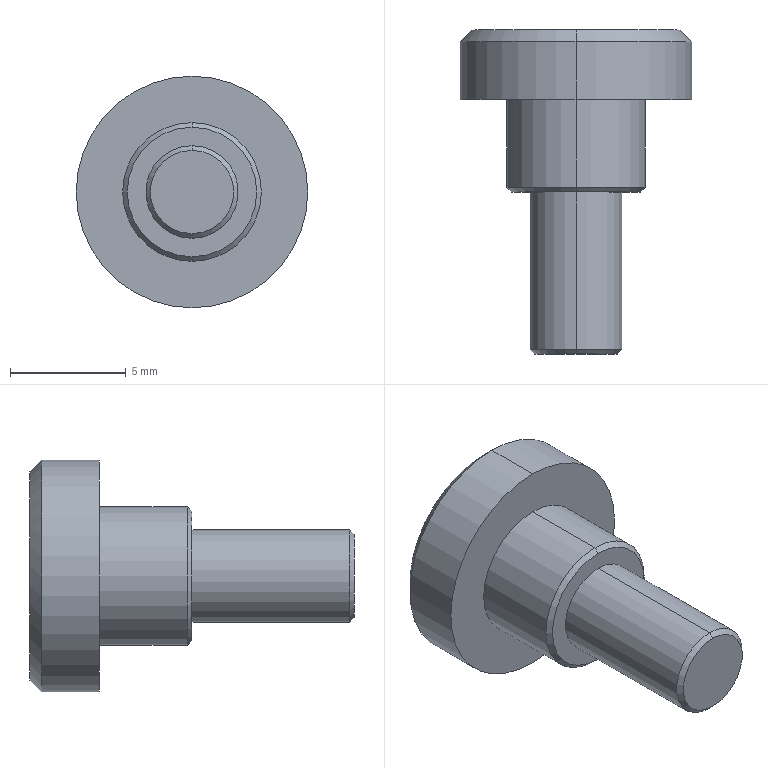Part | SolidWorks | features Chamfer 3, ICE 3, Extrusion 1 | 1 solid | 23 faces | box 10 x 14 x 10 mm | volume 408.891 mm3 | plane 11 | cone 6 | cylinder 6 | commonest cylinder face diameters 4 x2 6 x2 10 x2
STEP:
#1=CARTESIAN_POINT('',(0.,0.,-1.8));
#2=VERTEX_POINT('',#1);
#3=CARTESIAN_POINT('',(0.,0.,1.8));
#4=VERTEX_POINT('',#3);
#5=CARTESIAN_POINT('',(0.,0.,0.));
#6=DIRECTION('',(0.,-1.,0.));
#7=DIRECTION('',(0.,0.,1.));
#8=AXIS2_PLACEMENT_3D('',#5,#6,#7);
#9=CIRCLE('',#8,1.8);
#10=EDGE_CURVE('',#2,#4,#9,.T.);
#11=ORIENTED_EDGE('',*,*,#10,.F.);
#12=CARTESIAN_POINT('',(0.,0.2,-2.));
#13=VERTEX_POINT('',#12);
#14=CARTESIAN_POINT('',(0.,0.2,-2.));
#15=DIRECTION('',(0.,0.7071,-0.7071));
#16=VECTOR('',#15,1000.);
#17=LINE('',#14,#16);
#18=EDGE_CURVE('',#2,#13,#17,.T.);
#19=ORIENTED_EDGE('',*,*,#18,.T.);
#20=CARTESIAN_POINT('',(0.,0.2,2.));
#21=VERTEX_POINT('',#20);
#22=CARTESIAN_POINT('',(0.,0.2,0.));
#23=DIRECTION('',(0.,1.,0.));
#24=DIRECTION('',(0.,0.,1.));
#25=AXIS2_PLACEMENT_3D('',#22,#23,#24);
#26=CIRCLE('',#25,2.);
#27=EDGE_CURVE('',#21,#13,#26,.T.);
#28=ORIENTED_EDGE('',*,*,#27,.F.);
#29=CARTESIAN_POINT('',(0.,0.2,2.));
#30=DIRECTION('',(0.,0.7071,0.7071));
#31=VECTOR('',#30,1000.);
#32=LINE('',#29,#31);
#33=EDGE_CURVE('',#4,#21,#32,.T.);
#34=ORIENTED_EDGE('',*,*,#33,.F.);
#35=EDGE_LOOP('',(#11,#19,#28,#34));
#36=FACE_OUTER_BOUND('',#35,.T.);
#37=CARTESIAN_POINT('',(0.,0.2,0.));
#38=DIRECTION('',(0.,1.,0.));
#39=DIRECTION('',(0.,0.,1.));
#40=AXIS2_PLACEMENT_3D('',#37,#38,#39);
#41=CONICAL_SURFACE('',#40,2.,0.7854);
#42=ADVANCED_FACE('',(#36),#41,.T.);
#43=CARTESIAN_POINT('',(0.,7.,-2.8));
#44=VERTEX_POINT('',#43);
#45=CARTESIAN_POINT('',(0.,7.,2.8));
#46=VERTEX_POINT('',#45);
#47=CARTESIAN_POINT('',(0.,7.,0.));
#48=DIRECTION('',(0.,-1.,0.));
#49=DIRECTION('',(0.,0.,1.));
#50=AXIS2_PLACEMENT_3D('',#47,#48,#49);
#51=CIRCLE('',#50,2.8);
#52=EDGE_CURVE('',#44,#46,#51,.T.);
#53=ORIENTED_EDGE('',*,*,#52,.F.);
#54=CARTESIAN_POINT('',(0.,7.2,-3.));
#55=VERTEX_POINT('',#54);
#56=CARTESIAN_POINT('',(0.,7.2,-3.));
#57=DIRECTION('',(0.,0.7071,-0.7071));
#58=VECTOR('',#57,1000.);
#59=LINE('',#56,#58);
#60=EDGE_CURVE('',#44,#55,#59,.T.);
#61=ORIENTED_EDGE('',*,*,#60,.T.);
#62=CARTESIAN_POINT('',(0.,7.2,3.));
#63=VERTEX_POINT('',#62);
#64=CARTESIAN_POINT('',(0.,7.2,0.));
#65=DIRECTION('',(0.,1.,0.));
#66=DIRECTION('',(0.,0.,1.));
#67=AXIS2_PLACEMENT_3D('',#64,#65,#66);
#68=CIRCLE('',#67,3.);
#69=EDGE_CURVE('',#63,#55,#68,.T.);
#70=ORIENTED_EDGE('',*,*,#69,.F.);
#71=CARTESIAN_POINT('',(0.,7.2,3.));
#72=DIRECTION('',(0.,0.7071,0.7071));
#73=VECTOR('',#72,1000.);
#74=LINE('',#71,#73);
#75=EDGE_CURVE('',#46,#63,#74,.T.);
#76=ORIENTED_EDGE('',*,*,#75,.F.);
#77=EDGE_LOOP('',(#53,#61,#70,#76));
#78=FACE_OUTER_BOUND('',#77,.T.);
#79=CARTESIAN_POINT('',(0.,7.2,0.));
#80=DIRECTION('',(0.,1.,0.));
#81=DIRECTION('',(0.,0.,1.));
#82=AXIS2_PLACEMENT_3D('',#79,#80,#81);
#83=CONICAL_SURFACE('',#82,3.,0.7854);
#84=ADVANCED_FACE('',(#78),#83,.T.);
#85=CARTESIAN_POINT('',(0.,14.,4.5));
#86=VERTEX_POINT('',#85);
#87=CARTESIAN_POINT('',(0.,14.,-4.5));
#88=VERTEX_POINT('',#87);
#89=CARTESIAN_POINT('',(0.,14.,0.));
#90=DIRECTION('',(0.,1.,0.));
#91=DIRECTION('',(0.,0.,1.));
#92=AXIS2_PLACEMENT_3D('',#89,#90,#91);
#93=CIRCLE('',#92,4.5);
#94=EDGE_CURVE('',#86,#88,#93,.T.);
#95=ORIENTED_EDGE('',*,*,#94,.F.);
#96=CARTESIAN_POINT('',(0.,13.5,5.));
#97=VERTEX_POINT('',#96);
#98=CARTESIAN_POINT('',(0.,14.,4.5));
#99=DIRECTION('',(0.,-0.7071,0.7071));
#100=VECTOR('',#99,1000.);
#101=LINE('',#98,#100);
#102=EDGE_CURVE('',#86,#97,#101,.T.);
#103=ORIENTED_EDGE('',*,*,#102,.T.);
#104=CARTESIAN_POINT('',(0.,13.5,-5.));
#105=VERTEX_POINT('',#104);
#106=CARTESIAN_POINT('',(0.,13.5,0.));
#107=DIRECTION('',(0.,-1.,0.));
#108=DIRECTION('',(0.,0.,1.));
#109=AXIS2_PLACEMENT_3D('',#106,#107,#108);
#110=CIRCLE('',#109,5.);
#111=EDGE_CURVE('',#105,#97,#110,.T.);
#112=ORIENTED_EDGE('',*,*,#111,.F.);
#113=CARTESIAN_POINT('',(0.,14.,-4.5));
#114=DIRECTION('',(0.,-0.7071,-0.7071));
#115=VECTOR('',#114,1000.);
#116=LINE('',#113,#115);
#117=EDGE_CURVE('',#88,#105,#116,.T.);
#118=ORIENTED_EDGE('',*,*,#117,.F.);
#119=EDGE_LOOP('',(#95,#103,#112,#118));
#120=FACE_OUTER_BOUND('',#119,.T.);
#121=CARTESIAN_POINT('',(0.,14.,0.));
#122=DIRECTION('',(0.,-1.,0.));
#123=DIRECTION('',(0.,0.,-1.));
#124=AXIS2_PLACEMENT_3D('',#121,#122,#123);
#125=CONICAL_SURFACE('',#124,4.5,0.7854);
#126=ADVANCED_FACE('',(#120),#125,.T.);
#127=ORIENTED_EDGE('',*,*,#111,.T.);
#128=CARTESIAN_POINT('',(0.,11.,5.));
#129=VERTEX_POINT('',#128);
#130=CARTESIAN_POINT('',(0.,14.,5.));
#131=DIRECTION('',(0.,-1.,0.));
#132=VECTOR('',#131,1000.);
#133=LINE('',#130,#132);
#134=EDGE_CURVE('',#97,#129,#133,.T.);
#135=ORIENTED_EDGE('',*,*,#134,.T.);
#136=CARTESIAN_POINT('',(0.,11.,-5.));
#137=VERTEX_POINT('',#136);
#138=CARTESIAN_POINT('',(0.,11.,0.));
#139=DIRECTION('',(0.,1.,0.));
#140=DIRECTION('',(0.,0.,1.));
#141=AXIS2_PLACEMENT_3D('',#138,#139,#140);
#142=CIRCLE('',#141,5.);
#143=EDGE_CURVE('',#129,#137,#142,.T.);
#144=ORIENTED_EDGE('',*,*,#143,.T.);
#145=CARTESIAN_POINT('',(0.,14.,-5.));
#146=DIRECTION('',(0.,-1.,0.));
#147=VECTOR('',#146,1000.);
#148=LINE('',#145,#147);
#149=EDGE_CURVE('',#105,#137,#148,.T.);
#150=ORIENTED_EDGE('',*,*,#149,.F.);
#151=EDGE_LOOP('',(#127,#135,#144,#150));
#152=FACE_OUTER_BOUND('',#151,.T.);
#153=CARTESIAN_POINT('',(0.,14.,0.));
#154=DIRECTION('',(0.,-1.,0.));
#155=DIRECTION('',(0.,0.,-1.));
#156=AXIS2_PLACEMENT_3D('',#153,#154,#155);
#157=CYLINDRICAL_SURFACE('',#156,5.);
#158=ADVANCED_FACE('',(#152),#157,.T.);
#159=CARTESIAN_POINT('',(0.,11.,3.));
#160=VERTEX_POINT('',#159);
#161=CARTESIAN_POINT('',(0.,11.,-3.));
#162=VERTEX_POINT('',#161);
#163=CARTESIAN_POINT('',(0.,11.,0.));
#164=DIRECTION('',(0.,1.,0.));
#165=DIRECTION('',(0.,0.,1.));
#166=AXIS2_PLACEMENT_3D('',#163,#164,#165);
#167=CIRCLE('',#166,3.);
#168=EDGE_CURVE('',#160,#162,#167,.T.);
#169=ORIENTED_EDGE('',*,*,#168,.F.);
#170=CARTESIAN_POINT('',(0.,11.,3.));
#171=DIRECTION('',(0.,-1.,0.));
#172=VECTOR('',#171,1000.);
#173=LINE('',#170,#172);
#174=EDGE_CURVE('',#160,#63,#173,.T.);
#175=ORIENTED_EDGE('',*,*,#174,.T.);
#176=ORIENTED_EDGE('',*,*,#69,.T.);
#177=CARTESIAN_POINT('',(0.,11.,-3.));
#178=DIRECTION('',(0.,-1.,0.));
#179=VECTOR('',#178,1000.);
#180=LINE('',#177,#179);
#181=EDGE_CURVE('',#162,#55,#180,.T.);
#182=ORIENTED_EDGE('',*,*,#181,.F.);
#183=EDGE_LOOP('',(#169,#175,#176,#182));
#184=FACE_OUTER_BOUND('',#183,.T.);
#185=CARTESIAN_POINT('',(0.,11.,0.));
#186=DIRECTION('',(0.,-1.,0.));
#187=DIRECTION('',(0.,0.,-1.));
#188=AXIS2_PLACEMENT_3D('',#185,#186,#187);
#189=CYLINDRICAL_SURFACE('',#188,3.);
#190=ADVANCED_FACE('',(#184),#189,.T.);
#191=CARTESIAN_POINT('',(0.,7.,2.));
#192=VERTEX_POINT('',#191);
#193=CARTESIAN_POINT('',(0.,7.,-2.));
#194=VERTEX_POINT('',#193);
#195=CARTESIAN_POINT('',(0.,7.,0.));
#196=DIRECTION('',(0.,1.,0.));
#197=DIRECTION('',(0.,0.,1.));
#198=AXIS2_PLACEMENT_3D('',#195,#196,#197);
#199=CIRCLE('',#198,2.);
#200=EDGE_CURVE('',#192,#194,#199,.T.);
#201=ORIENTED_EDGE('',*,*,#200,.F.);
#202=CARTESIAN_POINT('',(0.,7.,2.));
#203=DIRECTION('',(0.,-1.,0.));
#204=VECTOR('',#203,1000.);
#205=LINE('',#202,#204);
#206=EDGE_CURVE('',#192,#21,#205,.T.);
#207=ORIENTED_EDGE('',*,*,#206,.T.);
#208=ORIENTED_EDGE('',*,*,#27,.T.);
#209=CARTESIAN_POINT('',(0.,7.,-2.));
#210=DIRECTION('',(0.,-1.,0.));
#211=VECTOR('',#210,1000.);
#212=LINE('',#209,#211);
#213=EDGE_CURVE('',#194,#13,#212,.T.);
#214=ORIENTED_EDGE('',*,*,#213,.F.);
#215=EDGE_LOOP('',(#201,#207,#208,#214));
#216=FACE_OUTER_BOUND('',#215,.T.);
#217=CARTESIAN_POINT('',(0.,7.,0.));
#218=DIRECTION('',(0.,-1.,0.));
#219=DIRECTION('',(0.,0.,-1.));
#220=AXIS2_PLACEMENT_3D('',#217,#218,#219);
#221=CYLINDRICAL_SURFACE('',#220,2.);
#222=ADVANCED_FACE('',(#216),#221,.T.);
#223=ORIENTED_EDGE('',*,*,#206,.F.);
#224=CARTESIAN_POINT('',(0.,7.,0.));
#225=DIRECTION('',(0.,1.,0.));
#226=DIRECTION('',(0.,0.,1.));
#227=AXIS2_PLACEMENT_3D('',#224,#225,#226);
#228=CIRCLE('',#227,2.);
#229=EDGE_CURVE('',#194,#192,#228,.T.);
#230=ORIENTED_EDGE('',*,*,#229,.F.);
#231=ORIENTED_EDGE('',*,*,#213,.T.);
#232=CARTESIAN_POINT('',(0.,0.2,0.));
#233=DIRECTION('',(0.,1.,0.));
#234=DIRECTION('',(0.,0.,1.));
#235=AXIS2_PLACEMENT_3D('',#232,#233,#234);
#236=CIRCLE('',#235,2.);
#237=EDGE_CURVE('',#13,#21,#236,.T.);
#238=ORIENTED_EDGE('',*,*,#237,.T.);
#239=EDGE_LOOP('',(#223,#230,#231,#238));
#240=FACE_OUTER_BOUND('',#239,.T.);
#241=CARTESIAN_POINT('',(0.,7.,0.));
#242=DIRECTION('',(0.,-1.,0.));
#243=DIRECTION('',(0.,0.,-1.));
#244=AXIS2_PLACEMENT_3D('',#241,#242,#243);
#245=CYLINDRICAL_SURFACE('',#244,2.);
#246=ADVANCED_FACE('',(#240),#245,.T.);
#247=CARTESIAN_POINT('',(0.,0.,0.));
#248=DIRECTION('',(0.,-1.,0.));
#249=DIRECTION('',(0.,0.,1.));
#250=AXIS2_PLACEMENT_3D('',#247,#248,#249);
#251=CIRCLE('',#250,1.8);
#252=EDGE_CURVE('',#4,#2,#251,.T.);
#253=ORIENTED_EDGE('',*,*,#252,.T.);
#254=ORIENTED_EDGE('',*,*,#10,.T.);
#255=EDGE_LOOP('',(#253,#254));
#256=FACE_OUTER_BOUND('',#255,.T.);
#257=CARTESIAN_POINT('',(0.,0.,0.));
#258=DIRECTION('',(0.,1.,0.));
#259=DIRECTION('',(0.,0.,1.));
#260=AXIS2_PLACEMENT_3D('',#257,#258,#259);
#261=PLANE('',#260);
#262=ADVANCED_FACE('',(#256),#261,.F.);
#263=CARTESIAN_POINT('',(0.,7.,0.));
#264=DIRECTION('',(0.,-1.,0.));
#265=DIRECTION('',(0.,0.,1.));
#266=AXIS2_PLACEMENT_3D('',#263,#264,#265);
#267=CIRCLE('',#266,2.8);
#268=EDGE_CURVE('',#46,#44,#267,.T.);
#269=ORIENTED_EDGE('',*,*,#268,.T.);
#270=ORIENTED_EDGE('',*,*,#52,.T.);
#271=EDGE_LOOP('',(#269,#270));
#272=FACE_OUTER_BOUND('',#271,.T.);
#273=ORIENTED_EDGE('',*,*,#229,.T.);
#274=ORIENTED_EDGE('',*,*,#200,.T.);
#275=EDGE_LOOP('',(#273,#274));
#276=FACE_BOUND('',#275,.T.);
#277=CARTESIAN_POINT('',(0.,7.,0.));
#278=DIRECTION('',(0.,1.,0.));
#279=DIRECTION('',(0.,0.,1.));
#280=AXIS2_PLACEMENT_3D('',#277,#278,#279);
#281=PLANE('',#280);
#282=ADVANCED_FACE('',(#272,#276),#281,.F.);
#283=ORIENTED_EDGE('',*,*,#174,.F.);
#284=CARTESIAN_POINT('',(0.,11.,0.));
#285=DIRECTION('',(0.,1.,0.));
#286=DIRECTION('',(0.,0.,1.));
#287=AXIS2_PLACEMENT_3D('',#284,#285,#286);
#288=CIRCLE('',#287,3.);
#289=EDGE_CURVE('',#162,#160,#288,.T.);
#290=ORIENTED_EDGE('',*,*,#289,.F.);
#291=ORIENTED_EDGE('',*,*,#181,.T.);
#292=CARTESIAN_POINT('',(0.,7.2,0.));
#293=DIRECTION('',(0.,1.,0.));
#294=DIRECTION('',(0.,0.,1.));
#295=AXIS2_PLACEMENT_3D('',#292,#293,#294);
#296=CIRCLE('',#295,3.);
#297=EDGE_CURVE('',#55,#63,#296,.T.);
#298=ORIENTED_EDGE('',*,*,#297,.T.);
#299=EDGE_LOOP('',(#283,#290,#291,#298));
#300=FACE_OUTER_BOUND('',#299,.T.);
#301=CARTESIAN_POINT('',(0.,11.,0.));
#302=DIRECTION('',(0.,-1.,0.));
#303=DIRECTION('',(0.,0.,-1.));
#304=AXIS2_PLACEMENT_3D('',#301,#302,#303);
#305=CYLINDRICAL_SURFACE('',#304,3.);
#306=ADVANCED_FACE('',(#300),#305,.T.);
#307=CARTESIAN_POINT('',(0.,11.,0.));
#308=DIRECTION('',(0.,1.,0.));
#309=DIRECTION('',(0.,0.,1.));
#310=AXIS2_PLACEMENT_3D('',#307,#308,#309);
#311=CIRCLE('',#310,5.);
#312=EDGE_CURVE('',#137,#129,#311,.T.);
#313=ORIENTED_EDGE('',*,*,#312,.F.);
#314=ORIENTED_EDGE('',*,*,#143,.F.);
#315=EDGE_LOOP('',(#313,#314));
#316=FACE_OUTER_BOUND('',#315,.T.);
#317=ORIENTED_EDGE('',*,*,#289,.T.);
#318=ORIENTED_EDGE('',*,*,#168,.T.);
#319=EDGE_LOOP('',(#317,#318));
#320=FACE_BOUND('',#319,.T.);
#321=CARTESIAN_POINT('',(0.,11.,0.));
#322=DIRECTION('',(0.,1.,0.));
#323=DIRECTION('',(0.,0.,1.));
#324=AXIS2_PLACEMENT_3D('',#321,#322,#323);
#325=PLANE('',#324);
#326=ADVANCED_FACE('',(#316,#320),#325,.F.);
#327=ORIENTED_EDGE('',*,*,#134,.F.);
#328=CARTESIAN_POINT('',(0.,13.5,0.));
#329=DIRECTION('',(0.,-1.,0.));
#330=DIRECTION('',(0.,0.,1.));
#331=AXIS2_PLACEMENT_3D('',#328,#329,#330);
#332=CIRCLE('',#331,5.);
#333=EDGE_CURVE('',#97,#105,#332,.T.);
#334=ORIENTED_EDGE('',*,*,#333,.T.);
#335=ORIENTED_EDGE('',*,*,#149,.T.);
#336=ORIENTED_EDGE('',*,*,#312,.T.);
#337=EDGE_LOOP('',(#327,#334,#335,#336));
#338=FACE_OUTER_BOUND('',#337,.T.);
#339=CARTESIAN_POINT('',(0.,14.,0.));
#340=DIRECTION('',(0.,-1.,0.));
#341=DIRECTION('',(0.,0.,-1.));
#342=AXIS2_PLACEMENT_3D('',#339,#340,#341);
#343=CYLINDRICAL_SURFACE('',#342,5.);
#344=ADVANCED_FACE('',(#338),#343,.T.);
#345=CARTESIAN_POINT('',(-0.6197,14.,1.617));
#346=VERTEX_POINT('',#345);
#347=CARTESIAN_POINT('',(1.091,14.,1.345));
#348=VERTEX_POINT('',#347);
#349=CARTESIAN_POINT('',(-0.6197,14.,1.617));
#350=DIRECTION('',(0.9876,0.,-0.157));
#351=VECTOR('',#350,1000.);
#352=LINE('',#349,#351);
#353=EDGE_CURVE('',#346,#348,#352,.T.);
#354=ORIENTED_EDGE('',*,*,#353,.F.);
#355=CARTESIAN_POINT('',(-1.711,14.,0.272));
#356=VERTEX_POINT('',#355);
#357=CARTESIAN_POINT('',(-1.711,14.,0.272));
#358=DIRECTION('',(0.6298,0.,0.7768));
#359=VECTOR('',#358,1000.);
#360=LINE('',#357,#359);
#361=EDGE_CURVE('',#356,#346,#360,.T.);
#362=ORIENTED_EDGE('',*,*,#361,.F.);
#363=CARTESIAN_POINT('',(-1.091,14.,-1.345));
#364=VERTEX_POINT('',#363);
#365=CARTESIAN_POINT('',(-1.091,14.,-1.345));
#366=DIRECTION('',(-0.3578,0.,0.9338));
#367=VECTOR('',#366,1000.);
#368=LINE('',#365,#367);
#369=EDGE_CURVE('',#364,#356,#368,.T.);
#370=ORIENTED_EDGE('',*,*,#369,.F.);
#371=CARTESIAN_POINT('',(0.6197,14.,-1.617));
#372=VERTEX_POINT('',#371);
#373=CARTESIAN_POINT('',(0.6197,14.,-1.617));
#374=DIRECTION('',(-0.9876,0.,0.157));
#375=VECTOR('',#374,1000.);
#376=LINE('',#373,#375);
#377=EDGE_CURVE('',#372,#364,#376,.T.);
#378=ORIENTED_EDGE('',*,*,#377,.F.);
#379=CARTESIAN_POINT('',(1.711,14.,-0.272));
#380=VERTEX_POINT('',#379);
#381=CARTESIAN_POINT('',(1.711,14.,-0.272));
#382=DIRECTION('',(-0.6298,0.,-0.7768));
#383=VECTOR('',#382,1000.);
#384=LINE('',#381,#383);
#385=EDGE_CURVE('',#380,#372,#384,.T.);
#386=ORIENTED_EDGE('',*,*,#385,.F.);
#387=CARTESIAN_POINT('',(1.091,14.,1.345));
#388=DIRECTION('',(0.3578,0.,-0.9338));
#389=VECTOR('',#388,1000.);
#390=LINE('',#387,#389);
#391=EDGE_CURVE('',#348,#380,#390,.T.);
#392=ORIENTED_EDGE('',*,*,#391,.F.);
#393=EDGE_LOOP('',(#354,#362,#370,#378,#386,#392));
#394=FACE_BOUND('',#393,.T.);
#395=CARTESIAN_POINT('',(0.,14.,0.));
#396=DIRECTION('',(0.,1.,0.));
#397=DIRECTION('',(0.,0.,1.));
#398=AXIS2_PLACEMENT_3D('',#395,#396,#397);
#399=CIRCLE('',#398,4.5);
#400=EDGE_CURVE('',#88,#86,#399,.T.);
#401=ORIENTED_EDGE('',*,*,#400,.T.);
#402=ORIENTED_EDGE('',*,*,#94,.T.);
#403=EDGE_LOOP('',(#401,#402));
#404=FACE_OUTER_BOUND('',#403,.T.);
#405=CARTESIAN_POINT('',(0.,14.,0.));
#406=DIRECTION('',(0.,1.,0.));
#407=DIRECTION('',(0.,0.,1.));
#408=AXIS2_PLACEMENT_3D('',#405,#406,#407);
#409=PLANE('',#408);
#410=ADVANCED_FACE('',(#394,#404),#409,.T.);
#411=ORIENTED_EDGE('',*,*,#102,.F.);
#412=ORIENTED_EDGE('',*,*,#400,.F.);
#413=ORIENTED_EDGE('',*,*,#117,.T.);
#414=ORIENTED_EDGE('',*,*,#333,.F.);
#415=EDGE_LOOP('',(#411,#412,#413,#414));
#416=FACE_OUTER_BOUND('',#415,.T.);
#417=CARTESIAN_POINT('',(0.,14.,0.));
#418=DIRECTION('',(0.,-1.,0.));
#419=DIRECTION('',(0.,0.,-1.));
#420=AXIS2_PLACEMENT_3D('',#417,#418,#419);
#421=CONICAL_SURFACE('',#420,4.5,0.7854);
#422=ADVANCED_FACE('',(#416),#421,.T.);
#423=ORIENTED_EDGE('',*,*,#60,.F.);
#424=ORIENTED_EDGE('',*,*,#268,.F.);
#425=ORIENTED_EDGE('',*,*,#75,.T.);
#426=ORIENTED_EDGE('',*,*,#297,.F.);
#427=EDGE_LOOP('',(#423,#424,#425,#426));
#428=FACE_OUTER_BOUND('',#427,.T.);
#429=CARTESIAN_POINT('',(0.,7.2,0.));
#430=DIRECTION('',(0.,1.,0.));
#431=DIRECTION('',(0.,0.,1.));
#432=AXIS2_PLACEMENT_3D('',#429,#430,#431);
#433=CONICAL_SURFACE('',#432,3.,0.7854);
#434=ADVANCED_FACE('',(#428),#433,.T.);
#435=ORIENTED_EDGE('',*,*,#18,.F.);
#436=ORIENTED_EDGE('',*,*,#252,.F.);
#437=ORIENTED_EDGE('',*,*,#33,.T.);
#438=ORIENTED_EDGE('',*,*,#237,.F.);
#439=EDGE_LOOP('',(#435,#436,#437,#438));
#440=FACE_OUTER_BOUND('',#439,.T.);
#441=CARTESIAN_POINT('',(0.,0.2,0.));
#442=DIRECTION('',(0.,1.,0.));
#443=DIRECTION('',(0.,0.,1.));
#444=AXIS2_PLACEMENT_3D('',#441,#442,#443);
#445=CONICAL_SURFACE('',#444,2.,0.7854);
#446=ADVANCED_FACE('',(#440),#445,.T.);
#447=ORIENTED_EDGE('',*,*,#353,.T.);
#448=CARTESIAN_POINT('',(1.091,11.,1.345));
#449=VERTEX_POINT('',#448);
#450=CARTESIAN_POINT('',(1.091,11.,1.345));
#451=DIRECTION('',(0.,1.,0.));
#452=VECTOR('',#451,1000.);
#453=LINE('',#450,#452);
#454=EDGE_CURVE('',#449,#348,#453,.T.);
#455=ORIENTED_EDGE('',*,*,#454,.F.);
#456=CARTESIAN_POINT('',(-0.6197,11.,1.617));
#457=VERTEX_POINT('',#456);
#458=CARTESIAN_POINT('',(-0.6197,11.,1.617));
#459=DIRECTION('',(0.9876,0.,-0.157));
#460=VECTOR('',#459,1000.);
#461=LINE('',#458,#460);
#462=EDGE_CURVE('',#457,#449,#461,.T.);
#463=ORIENTED_EDGE('',*,*,#462,.F.);
#464=CARTESIAN_POINT('',(-0.6197,11.,1.617));
#465=DIRECTION('',(0.,1.,0.));
#466=VECTOR('',#465,1000.);
#467=LINE('',#464,#466);
#468=EDGE_CURVE('',#457,#346,#467,.T.);
#469=ORIENTED_EDGE('',*,*,#468,.T.);
#470=EDGE_LOOP('',(#447,#455,#463,#469));
#471=FACE_OUTER_BOUND('',#470,.T.);
#472=CARTESIAN_POINT('',(-0.6197,11.,1.617));
#473=DIRECTION('',(0.157,0.,0.9876));
#474=DIRECTION('',(0.9876,0.,-0.157));
#475=AXIS2_PLACEMENT_3D('',#472,#473,#474);
#476=PLANE('',#475);
#477=ADVANCED_FACE('',(#471),#476,.F.);
#478=ORIENTED_EDGE('',*,*,#361,.T.);
#479=ORIENTED_EDGE('',*,*,#468,.F.);
#480=CARTESIAN_POINT('',(-1.711,11.,0.272));
#481=VERTEX_POINT('',#480);
#482=CARTESIAN_POINT('',(-1.711,11.,0.272));
#483=DIRECTION('',(0.6298,0.,0.7768));
#484=VECTOR('',#483,1000.);
#485=LINE('',#482,#484);
#486=EDGE_CURVE('',#481,#457,#485,.T.);
#487=ORIENTED_EDGE('',*,*,#486,.F.);
#488=CARTESIAN_POINT('',(-1.711,11.,0.272));
#489=DIRECTION('',(0.,1.,0.));
#490=VECTOR('',#489,1000.);
#491=LINE('',#488,#490);
#492=EDGE_CURVE('',#481,#356,#491,.T.);
#493=ORIENTED_EDGE('',*,*,#492,.T.);
#494=EDGE_LOOP('',(#478,#479,#487,#493));
#495=FACE_OUTER_BOUND('',#494,.T.);
#496=CARTESIAN_POINT('',(-1.711,11.,0.272));
#497=DIRECTION('',(-0.7768,0.,0.6298));
#498=DIRECTION('',(0.6298,0.,0.7768));
#499=AXIS2_PLACEMENT_3D('',#496,#497,#498);
#500=PLANE('',#499);
#501=ADVANCED_FACE('',(#495),#500,.F.);
#502=ORIENTED_EDGE('',*,*,#369,.T.);
#503=ORIENTED_EDGE('',*,*,#492,.F.);
#504=CARTESIAN_POINT('',(-1.091,11.,-1.345));
#505=VERTEX_POINT('',#504);
#506=CARTESIAN_POINT('',(-1.091,11.,-1.345));
#507=DIRECTION('',(-0.3578,0.,0.9338));
#508=VECTOR('',#507,1000.);
#509=LINE('',#506,#508);
#510=EDGE_CURVE('',#505,#481,#509,.T.);
#511=ORIENTED_EDGE('',*,*,#510,.F.);
#512=CARTESIAN_POINT('',(-1.091,11.,-1.345));
#513=DIRECTION('',(0.,1.,0.));
#514=VECTOR('',#513,1000.);
#515=LINE('',#512,#514);
#516=EDGE_CURVE('',#505,#364,#515,.T.);
#517=ORIENTED_EDGE('',*,*,#516,.T.);
#518=EDGE_LOOP('',(#502,#503,#511,#517));
#519=FACE_OUTER_BOUND('',#518,.T.);
#520=CARTESIAN_POINT('',(-1.091,11.,-1.345));
#521=DIRECTION('',(-0.9338,0.,-0.3578));
#522=DIRECTION('',(-0.3578,0.,0.9338));
#523=AXIS2_PLACEMENT_3D('',#520,#521,#522);
#524=PLANE('',#523);
#525=ADVANCED_FACE('',(#519),#524,.F.);
#526=ORIENTED_EDGE('',*,*,#377,.T.);
#527=ORIENTED_EDGE('',*,*,#516,.F.);
#528=CARTESIAN_POINT('',(0.6197,11.,-1.617));
#529=VERTEX_POINT('',#528);
#530=CARTESIAN_POINT('',(0.6197,11.,-1.617));
#531=DIRECTION('',(-0.9876,0.,0.157));
#532=VECTOR('',#531,1000.);
#533=LINE('',#530,#532);
#534=EDGE_CURVE('',#529,#505,#533,.T.);
#535=ORIENTED_EDGE('',*,*,#534,.F.);
#536=CARTESIAN_POINT('',(0.6197,11.,-1.617));
#537=DIRECTION('',(0.,1.,0.));
#538=VECTOR('',#537,1000.);
#539=LINE('',#536,#538);
#540=EDGE_CURVE('',#529,#372,#539,.T.);
#541=ORIENTED_EDGE('',*,*,#540,.T.);
#542=EDGE_LOOP('',(#526,#527,#535,#541));
#543=FACE_OUTER_BOUND('',#542,.T.);
#544=CARTESIAN_POINT('',(0.6197,11.,-1.617));
#545=DIRECTION('',(-0.157,0.,-0.9876));
#546=DIRECTION('',(-0.9876,0.,0.157));
#547=AXIS2_PLACEMENT_3D('',#544,#545,#546);
#548=PLANE('',#547);
#549=ADVANCED_FACE('',(#543),#548,.F.);
#550=ORIENTED_EDGE('',*,*,#385,.T.);
#551=ORIENTED_EDGE('',*,*,#540,.F.);
#552=CARTESIAN_POINT('',(1.711,11.,-0.272));
#553=VERTEX_POINT('',#552);
#554=CARTESIAN_POINT('',(1.711,11.,-0.272));
#555=DIRECTION('',(-0.6298,0.,-0.7768));
#556=VECTOR('',#555,1000.);
#557=LINE('',#554,#556);
#558=EDGE_CURVE('',#553,#529,#557,.T.);
#559=ORIENTED_EDGE('',*,*,#558,.F.);
#560=CARTESIAN_POINT('',(1.711,11.,-0.272));
#561=DIRECTION('',(0.,1.,0.));
#562=VECTOR('',#561,1000.);
#563=LINE('',#560,#562);
#564=EDGE_CURVE('',#553,#380,#563,.T.);
#565=ORIENTED_EDGE('',*,*,#564,.T.);
#566=EDGE_LOOP('',(#550,#551,#559,#565));
#567=FACE_OUTER_BOUND('',#566,.T.);
#568=CARTESIAN_POINT('',(1.711,11.,-0.272));
#569=DIRECTION('',(0.7768,0.,-0.6298));
#570=DIRECTION('',(-0.6298,0.,-0.7768));
#571=AXIS2_PLACEMENT_3D('',#568,#569,#570);
#572=PLANE('',#571);
#573=ADVANCED_FACE('',(#567),#572,.F.);
#574=ORIENTED_EDGE('',*,*,#391,.T.);
#575=ORIENTED_EDGE('',*,*,#564,.F.);
#576=CARTESIAN_POINT('',(1.091,11.,1.345));
#577=DIRECTION('',(0.3578,0.,-0.9338));
#578=VECTOR('',#577,1000.);
#579=LINE('',#576,#578);
#580=EDGE_CURVE('',#449,#553,#579,.T.);
#581=ORIENTED_EDGE('',*,*,#580,.F.);
#582=ORIENTED_EDGE('',*,*,#454,.T.);
#583=EDGE_LOOP('',(#574,#575,#581,#582));
#584=FACE_OUTER_BOUND('',#583,.T.);
#585=CARTESIAN_POINT('',(1.091,11.,1.345));
#586=DIRECTION('',(0.9338,0.,0.3578));
#587=DIRECTION('',(0.3578,0.,-0.9338));
#588=AXIS2_PLACEMENT_3D('',#585,#586,#587);
#589=PLANE('',#588);
#590=ADVANCED_FACE('',(#584),#589,.F.);
#591=ORIENTED_EDGE('',*,*,#462,.T.);
#592=ORIENTED_EDGE('',*,*,#580,.T.);
#593=ORIENTED_EDGE('',*,*,#558,.T.);
#594=ORIENTED_EDGE('',*,*,#534,.T.);
#595=ORIENTED_EDGE('',*,*,#510,.T.);
#596=ORIENTED_EDGE('',*,*,#486,.T.);
#597=EDGE_LOOP('',(#591,#592,#593,#594,#595,#596));
#598=FACE_OUTER_BOUND('',#597,.T.);
#599=CARTESIAN_POINT('',(0.,11.,0.));
#600=DIRECTION('',(0.,1.,0.));
#601=DIRECTION('',(0.,0.,1.));
#602=AXIS2_PLACEMENT_3D('',#599,#600,#601);
#603=PLANE('',#602);
#604=ADVANCED_FACE('',(#598),#603,.T.);
#605=CLOSED_SHELL('',(#42,#84,#126,#158,#190,#222,#246,#262,#282,#306,#326,#344,#410,#422,#434,#446,#477,#501,#525,#549,#573,#590,#604));
#606=MANIFOLD_SOLID_BREP('',#605);
#607=CARTESIAN_POINT('',(0.,0.,0.));
#608=DIRECTION('',(0.,0.,1.));
#609=DIRECTION('',(1.,0.,0.));
#610=AXIS2_PLACEMENT_3D('',#607,#608,#609);
#611=(LENGTH_UNIT()NAMED_UNIT(*)SI_UNIT(.MILLI.,.METRE.));
#612=UNCERTAINTY_MEASURE_WITH_UNIT(LENGTH_MEASURE(0.00001),#611,'','');
#613=(NAMED_UNIT(*)PLANE_ANGLE_UNIT()SI_UNIT($,.RADIAN.));
#614=(NAMED_UNIT(*)SI_UNIT($,.STERADIAN.)SOLID_ANGLE_UNIT());
#615=(GEOMETRIC_REPRESENTATION_CONTEXT(3)GLOBAL_UNCERTAINTY_ASSIGNED_CONTEXT((#612))GLOBAL_UNIT_ASSIGNED_CONTEXT((#611,#613,#614))REPRESENTATION_CONTEXT('',''));
#616=ADVANCED_BREP_SHAPE_REPRESENTATION('',(#606,#610),#615);